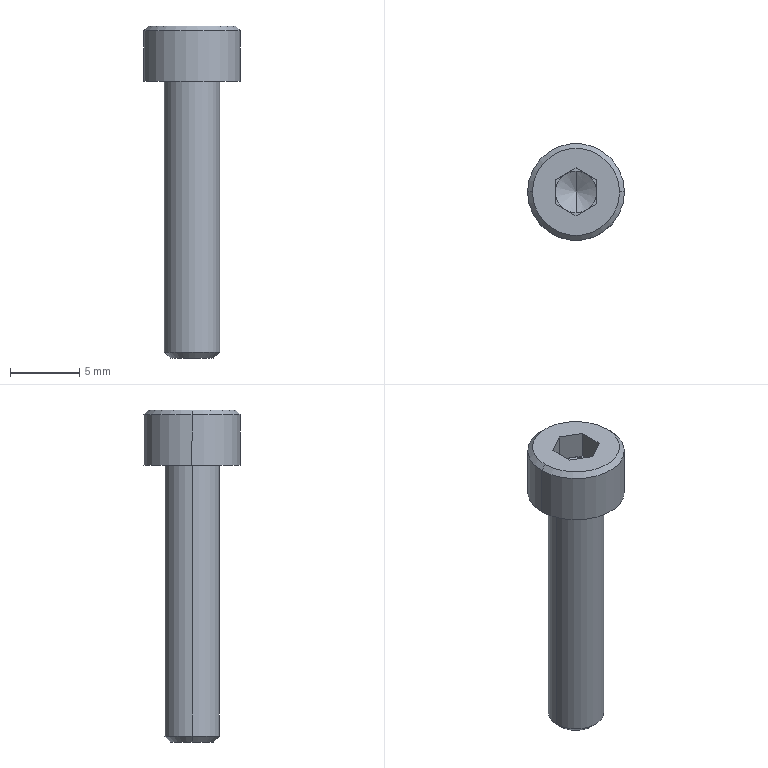Part | NX | features BREP 1 | 1 solid | 25 faces | box 7 x 7 x 24 mm | volume 385.258 mm3 | plane 15 | cone 6 | cylinder 4 | commonest cylinder face diameters 4 x2 7 x2
STEP:
#1=CARTESIAN_POINT('',(0.,-1.5,2.));
#2=VERTEX_POINT('',#1);
#3=CARTESIAN_POINT('',(0.,0.,1.134));
#4=VERTEX_POINT('',#3);
#5=CARTESIAN_POINT('',(0.,0.,1.134));
#6=DIRECTION('',(0.,-0.866,0.5));
#7=VECTOR('',#6,1000.);
#8=LINE('',#5,#7);
#9=EDGE_CURVE('',#2,#4,#8,.F.);
#10=ORIENTED_EDGE('',*,*,#9,.T.);
#11=CARTESIAN_POINT('',(0.,1.5,2.));
#12=VERTEX_POINT('',#11);
#13=CARTESIAN_POINT('',(0.,0.,1.134));
#14=DIRECTION('',(0.,0.866,0.5));
#15=VECTOR('',#14,1000.);
#16=LINE('',#13,#15);
#17=EDGE_CURVE('',#12,#4,#16,.F.);
#18=ORIENTED_EDGE('',*,*,#17,.F.);
#19=CARTESIAN_POINT('',(-0.75,1.299,2.));
#20=VERTEX_POINT('',#19);
#21=CARTESIAN_POINT('',(0.,0.,2.));
#22=DIRECTION('',(0.,0.,1.));
#23=DIRECTION('',(0.,-1.,0.));
#24=AXIS2_PLACEMENT_3D('',#21,#22,#23);
#25=CIRCLE('',#24,1.5);
#26=EDGE_CURVE('',#12,#20,#25,.T.);
#27=ORIENTED_EDGE('',*,*,#26,.T.);
#28=CARTESIAN_POINT('',(-1.5,0.,2.));
#29=VERTEX_POINT('',#28);
#30=CARTESIAN_POINT('',(0.,0.,2.));
#31=DIRECTION('',(0.,0.,1.));
#32=DIRECTION('',(0.,-1.,0.));
#33=AXIS2_PLACEMENT_3D('',#30,#31,#32);
#34=CIRCLE('',#33,1.5);
#35=EDGE_CURVE('',#20,#29,#34,.T.);
#36=ORIENTED_EDGE('',*,*,#35,.T.);
#37=CARTESIAN_POINT('',(-0.75,-1.299,2.));
#38=VERTEX_POINT('',#37);
#39=CARTESIAN_POINT('',(0.,0.,2.));
#40=DIRECTION('',(0.,0.,1.));
#41=DIRECTION('',(0.,-1.,0.));
#42=AXIS2_PLACEMENT_3D('',#39,#40,#41);
#43=CIRCLE('',#42,1.5);
#44=EDGE_CURVE('',#29,#38,#43,.T.);
#45=ORIENTED_EDGE('',*,*,#44,.T.);
#46=CARTESIAN_POINT('',(0.,0.,2.));
#47=DIRECTION('',(0.,0.,1.));
#48=DIRECTION('',(0.,-1.,0.));
#49=AXIS2_PLACEMENT_3D('',#46,#47,#48);
#50=CIRCLE('',#49,1.5);
#51=EDGE_CURVE('',#38,#2,#50,.T.);
#52=ORIENTED_EDGE('',*,*,#51,.T.);
#53=EDGE_LOOP('',(#10,#18,#27,#36,#45,#52));
#54=FACE_BOUND('',#53,.T.);
#55=CARTESIAN_POINT('',(0.,0.,1001.134));
#56=DIRECTION('',(0.,0.,1.));
#57=DIRECTION('',(0.,1.,0.));
#58=AXIS2_PLACEMENT_3D('',#55,#56,#57);
#59=CONICAL_SURFACE('',#58,1732.051,1.047);
#60=ADVANCED_FACE('',(#54),#59,.F.);
#61=CARTESIAN_POINT('',(3.5,0.,0.));
#62=VERTEX_POINT('',#61);
#63=CARTESIAN_POINT('',(-3.5,0.,0.));
#64=VERTEX_POINT('',#63);
#65=CARTESIAN_POINT('',(0.,0.,0.));
#66=DIRECTION('',(0.,0.,1.));
#67=DIRECTION('',(1.,0.,0.));
#68=AXIS2_PLACEMENT_3D('',#65,#66,#67);
#69=CIRCLE('',#68,3.5);
#70=EDGE_CURVE('',#62,#64,#69,.T.);
#71=ORIENTED_EDGE('',*,*,#70,.T.);
#72=CARTESIAN_POINT('',(-3.5,0.,3.65));
#73=VERTEX_POINT('',#72);
#74=CARTESIAN_POINT('',(-3.5,0.,0.));
#75=DIRECTION('',(0.,0.,1.));
#76=VECTOR('',#75,1000.);
#77=LINE('',#74,#76);
#78=EDGE_CURVE('',#64,#73,#77,.T.);
#79=ORIENTED_EDGE('',*,*,#78,.T.);
#80=CARTESIAN_POINT('',(3.5,0.,3.65));
#81=VERTEX_POINT('',#80);
#82=CARTESIAN_POINT('',(0.,0.,3.65));
#83=DIRECTION('',(0.,0.,1.));
#84=DIRECTION('',(1.,0.,0.));
#85=AXIS2_PLACEMENT_3D('',#82,#83,#84);
#86=CIRCLE('',#85,3.5);
#87=EDGE_CURVE('',#81,#73,#86,.T.);
#88=ORIENTED_EDGE('',*,*,#87,.F.);
#89=CARTESIAN_POINT('',(3.5,0.,0.));
#90=DIRECTION('',(0.,0.,1.));
#91=VECTOR('',#90,1000.);
#92=LINE('',#89,#91);
#93=EDGE_CURVE('',#62,#81,#92,.T.);
#94=ORIENTED_EDGE('',*,*,#93,.F.);
#95=EDGE_LOOP('',(#71,#79,#88,#94));
#96=FACE_BOUND('',#95,.T.);
#97=CARTESIAN_POINT('',(0.,0.,0.));
#98=DIRECTION('',(0.,0.,1.));
#99=DIRECTION('',(-1.,0.,0.));
#100=AXIS2_PLACEMENT_3D('',#97,#98,#99);
#101=CYLINDRICAL_SURFACE('',#100,3.5);
#102=ADVANCED_FACE('',(#96),#101,.T.);
#103=CARTESIAN_POINT('',(3.15,0.,4.));
#104=VERTEX_POINT('',#103);
#105=CARTESIAN_POINT('',(-3.15,0.,4.));
#106=VERTEX_POINT('',#105);
#107=CARTESIAN_POINT('',(0.,0.,4.));
#108=DIRECTION('',(0.,0.,1.));
#109=DIRECTION('',(1.,0.,0.));
#110=AXIS2_PLACEMENT_3D('',#107,#108,#109);
#111=CIRCLE('',#110,3.15);
#112=EDGE_CURVE('',#104,#106,#111,.T.);
#113=ORIENTED_EDGE('',*,*,#112,.F.);
#114=CARTESIAN_POINT('',(3.5,0.,3.65));
#115=DIRECTION('',(0.7071,0.,-0.7071));
#116=VECTOR('',#115,1000.);
#117=LINE('',#114,#116);
#118=EDGE_CURVE('',#81,#104,#117,.F.);
#119=ORIENTED_EDGE('',*,*,#118,.F.);
#120=ORIENTED_EDGE('',*,*,#87,.T.);
#121=CARTESIAN_POINT('',(-3.5,0.,3.65));
#122=DIRECTION('',(-0.7071,0.,-0.7071));
#123=VECTOR('',#122,1000.);
#124=LINE('',#121,#123);
#125=EDGE_CURVE('',#73,#106,#124,.F.);
#126=ORIENTED_EDGE('',*,*,#125,.T.);
#127=EDGE_LOOP('',(#113,#119,#120,#126));
#128=FACE_BOUND('',#127,.T.);
#129=CARTESIAN_POINT('',(0.,0.,3.65));
#130=DIRECTION('',(0.,0.,-1.));
#131=DIRECTION('',(1.,0.,0.));
#132=AXIS2_PLACEMENT_3D('',#129,#130,#131);
#133=CONICAL_SURFACE('',#132,3.5,0.7854);
#134=ADVANCED_FACE('',(#128),#133,.T.);
#135=CARTESIAN_POINT('',(1.571,0.,-20.));
#136=VERTEX_POINT('',#135);
#137=CARTESIAN_POINT('',(-1.571,0.,-20.));
#138=VERTEX_POINT('',#137);
#139=CARTESIAN_POINT('',(0.,0.,-20.));
#140=DIRECTION('',(0.,0.,1.));
#141=DIRECTION('',(1.,0.,0.));
#142=AXIS2_PLACEMENT_3D('',#139,#140,#141);
#143=CIRCLE('',#142,1.571);
#144=EDGE_CURVE('',#136,#138,#143,.T.);
#145=ORIENTED_EDGE('',*,*,#144,.T.);
#146=CARTESIAN_POINT('',(-2.,0.,-19.57));
#147=VERTEX_POINT('',#146);
#148=CARTESIAN_POINT('',(-1.571,0.,-20.));
#149=DIRECTION('',(-0.7071,0.,0.7071));
#150=VECTOR('',#149,1000.);
#151=LINE('',#148,#150);
#152=EDGE_CURVE('',#138,#147,#151,.T.);
#153=ORIENTED_EDGE('',*,*,#152,.T.);
#154=CARTESIAN_POINT('',(2.,0.,-19.57));
#155=VERTEX_POINT('',#154);
#156=CARTESIAN_POINT('',(0.,0.,-19.57));
#157=DIRECTION('',(0.,0.,1.));
#158=DIRECTION('',(1.,0.,0.));
#159=AXIS2_PLACEMENT_3D('',#156,#157,#158);
#160=CIRCLE('',#159,2.);
#161=EDGE_CURVE('',#155,#147,#160,.T.);
#162=ORIENTED_EDGE('',*,*,#161,.F.);
#163=CARTESIAN_POINT('',(1.571,0.,-20.));
#164=DIRECTION('',(0.7071,0.,0.7071));
#165=VECTOR('',#164,1000.);
#166=LINE('',#163,#165);
#167=EDGE_CURVE('',#136,#155,#166,.T.);
#168=ORIENTED_EDGE('',*,*,#167,.F.);
#169=EDGE_LOOP('',(#145,#153,#162,#168));
#170=FACE_BOUND('',#169,.T.);
#171=CARTESIAN_POINT('',(0.,0.,-20.));
#172=DIRECTION('',(0.,0.,1.));
#173=DIRECTION('',(-1.,0.,0.));
#174=AXIS2_PLACEMENT_3D('',#171,#172,#173);
#175=CONICAL_SURFACE('',#174,1.571,0.7854);
#176=ADVANCED_FACE('',(#170),#175,.T.);
#177=ORIENTED_EDGE('',*,*,#161,.T.);
#178=CARTESIAN_POINT('',(-2.,0.,0.));
#179=VERTEX_POINT('',#178);
#180=CARTESIAN_POINT('',(-2.,0.,-20.));
#181=DIRECTION('',(0.,0.,1.));
#182=VECTOR('',#181,1000.);
#183=LINE('',#180,#182);
#184=EDGE_CURVE('',#147,#179,#183,.T.);
#185=ORIENTED_EDGE('',*,*,#184,.T.);
#186=CARTESIAN_POINT('',(2.,0.,0.));
#187=VERTEX_POINT('',#186);
#188=CARTESIAN_POINT('',(0.,0.,0.));
#189=DIRECTION('',(0.,0.,1.));
#190=DIRECTION('',(1.,0.,0.));
#191=AXIS2_PLACEMENT_3D('',#188,#189,#190);
#192=CIRCLE('',#191,2.);
#193=EDGE_CURVE('',#187,#179,#192,.T.);
#194=ORIENTED_EDGE('',*,*,#193,.F.);
#195=CARTESIAN_POINT('',(2.,0.,-20.));
#196=DIRECTION('',(0.,0.,1.));
#197=VECTOR('',#196,1000.);
#198=LINE('',#195,#197);
#199=EDGE_CURVE('',#155,#187,#198,.T.);
#200=ORIENTED_EDGE('',*,*,#199,.F.);
#201=EDGE_LOOP('',(#177,#185,#194,#200));
#202=FACE_BOUND('',#201,.T.);
#203=CARTESIAN_POINT('',(0.,0.,-20.));
#204=DIRECTION('',(0.,0.,1.));
#205=DIRECTION('',(-1.,0.,0.));
#206=AXIS2_PLACEMENT_3D('',#203,#204,#205);
#207=CYLINDRICAL_SURFACE('',#206,2.);
#208=ADVANCED_FACE('',(#202),#207,.T.);
#209=CARTESIAN_POINT('',(0.75,-1.299,2.));
#210=VERTEX_POINT('',#209);
#211=CARTESIAN_POINT('',(1.5,0.,2.));
#212=VERTEX_POINT('',#211);
#213=CARTESIAN_POINT('',(0.,0.,2.));
#214=DIRECTION('',(0.,0.,1.));
#215=DIRECTION('',(0.,-1.,0.));
#216=AXIS2_PLACEMENT_3D('',#213,#214,#215);
#217=CIRCLE('',#216,1.5);
#218=EDGE_CURVE('',#210,#212,#217,.T.);
#219=ORIENTED_EDGE('',*,*,#218,.F.);
#220=CARTESIAN_POINT('',(1.5,-0.866,2.));
#221=VERTEX_POINT('',#220);
#222=CARTESIAN_POINT('',(0.,-1.732,2.));
#223=DIRECTION('',(0.866,0.5,0.));
#224=VECTOR('',#223,1000.);
#225=LINE('',#222,#224);
#226=EDGE_CURVE('',#210,#221,#225,.T.);
#227=ORIENTED_EDGE('',*,*,#226,.T.);
#228=CARTESIAN_POINT('',(1.5,-0.866,2.));
#229=DIRECTION('',(0.,1.,0.));
#230=VECTOR('',#229,1000.);
#231=LINE('',#228,#230);
#232=EDGE_CURVE('',#221,#212,#231,.T.);
#233=ORIENTED_EDGE('',*,*,#232,.T.);
#234=EDGE_LOOP('',(#219,#227,#233));
#235=FACE_BOUND('',#234,.T.);
#236=CARTESIAN_POINT('',(0.,0.,2.));
#237=DIRECTION('',(0.,0.,1.));
#238=DIRECTION('',(-1.,0.,0.));
#239=AXIS2_PLACEMENT_3D('',#236,#237,#238);
#240=PLANE('',#239);
#241=ADVANCED_FACE('',(#235),#240,.T.);
#242=CARTESIAN_POINT('',(0.75,1.299,2.));
#243=VERTEX_POINT('',#242);
#244=CARTESIAN_POINT('',(0.,0.,2.));
#245=DIRECTION('',(0.,0.,1.));
#246=DIRECTION('',(0.,-1.,0.));
#247=AXIS2_PLACEMENT_3D('',#244,#245,#246);
#248=CIRCLE('',#247,1.5);
#249=EDGE_CURVE('',#212,#243,#248,.T.);
#250=ORIENTED_EDGE('',*,*,#249,.F.);
#251=CARTESIAN_POINT('',(1.5,0.866,2.));
#252=VERTEX_POINT('',#251);
#253=CARTESIAN_POINT('',(1.5,-0.866,2.));
#254=DIRECTION('',(0.,1.,0.));
#255=VECTOR('',#254,1000.);
#256=LINE('',#253,#255);
#257=EDGE_CURVE('',#212,#252,#256,.T.);
#258=ORIENTED_EDGE('',*,*,#257,.T.);
#259=CARTESIAN_POINT('',(1.5,0.866,2.));
#260=DIRECTION('',(-0.866,0.5,0.));
#261=VECTOR('',#260,1000.);
#262=LINE('',#259,#261);
#263=EDGE_CURVE('',#252,#243,#262,.T.);
#264=ORIENTED_EDGE('',*,*,#263,.T.);
#265=EDGE_LOOP('',(#250,#258,#264));
#266=FACE_BOUND('',#265,.T.);
#267=CARTESIAN_POINT('',(0.,0.,2.));
#268=DIRECTION('',(0.,0.,1.));
#269=DIRECTION('',(-1.,0.,0.));
#270=AXIS2_PLACEMENT_3D('',#267,#268,#269);
#271=PLANE('',#270);
#272=ADVANCED_FACE('',(#266),#271,.T.);
#273=CARTESIAN_POINT('',(0.,0.,2.));
#274=DIRECTION('',(0.,0.,1.));
#275=DIRECTION('',(0.,-1.,0.));
#276=AXIS2_PLACEMENT_3D('',#273,#274,#275);
#277=CIRCLE('',#276,1.5);
#278=EDGE_CURVE('',#243,#12,#277,.T.);
#279=ORIENTED_EDGE('',*,*,#278,.F.);
#280=CARTESIAN_POINT('',(0.,1.732,2.));
#281=VERTEX_POINT('',#280);
#282=CARTESIAN_POINT('',(1.5,0.866,2.));
#283=DIRECTION('',(-0.866,0.5,0.));
#284=VECTOR('',#283,1000.);
#285=LINE('',#282,#284);
#286=EDGE_CURVE('',#243,#281,#285,.T.);
#287=ORIENTED_EDGE('',*,*,#286,.T.);
#288=CARTESIAN_POINT('',(0.,1.732,2.));
#289=DIRECTION('',(-0.866,-0.5,0.));
#290=VECTOR('',#289,1000.);
#291=LINE('',#288,#290);
#292=EDGE_CURVE('',#281,#20,#291,.T.);
#293=ORIENTED_EDGE('',*,*,#292,.T.);
#294=ORIENTED_EDGE('',*,*,#26,.F.);
#295=EDGE_LOOP('',(#279,#287,#293,#294));
#296=FACE_BOUND('',#295,.T.);
#297=CARTESIAN_POINT('',(0.,0.,2.));
#298=DIRECTION('',(0.,0.,1.));
#299=DIRECTION('',(-1.,0.,0.));
#300=AXIS2_PLACEMENT_3D('',#297,#298,#299);
#301=PLANE('',#300);
#302=ADVANCED_FACE('',(#296),#301,.T.);
#303=ORIENTED_EDGE('',*,*,#35,.F.);
#304=CARTESIAN_POINT('',(-1.5,0.866,2.));
#305=VERTEX_POINT('',#304);
#306=CARTESIAN_POINT('',(0.,1.732,2.));
#307=DIRECTION('',(-0.866,-0.5,0.));
#308=VECTOR('',#307,1000.);
#309=LINE('',#306,#308);
#310=EDGE_CURVE('',#20,#305,#309,.T.);
#311=ORIENTED_EDGE('',*,*,#310,.T.);
#312=CARTESIAN_POINT('',(-1.5,0.866,2.));
#313=DIRECTION('',(0.,-1.,0.));
#314=VECTOR('',#313,1000.);
#315=LINE('',#312,#314);
#316=EDGE_CURVE('',#305,#29,#315,.T.);
#317=ORIENTED_EDGE('',*,*,#316,.T.);
#318=EDGE_LOOP('',(#303,#311,#317));
#319=FACE_BOUND('',#318,.T.);
#320=CARTESIAN_POINT('',(0.,0.,2.));
#321=DIRECTION('',(0.,0.,1.));
#322=DIRECTION('',(-1.,0.,0.));
#323=AXIS2_PLACEMENT_3D('',#320,#321,#322);
#324=PLANE('',#323);
#325=ADVANCED_FACE('',(#319),#324,.T.);
#326=ORIENTED_EDGE('',*,*,#44,.F.);
#327=CARTESIAN_POINT('',(-1.5,-0.866,2.));
#328=VERTEX_POINT('',#327);
#329=CARTESIAN_POINT('',(-1.5,0.866,2.));
#330=DIRECTION('',(0.,-1.,0.));
#331=VECTOR('',#330,1000.);
#332=LINE('',#329,#331);
#333=EDGE_CURVE('',#29,#328,#332,.T.);
#334=ORIENTED_EDGE('',*,*,#333,.T.);
#335=CARTESIAN_POINT('',(-1.5,-0.866,2.));
#336=DIRECTION('',(0.866,-0.5,0.));
#337=VECTOR('',#336,1000.);
#338=LINE('',#335,#337);
#339=EDGE_CURVE('',#328,#38,#338,.T.);
#340=ORIENTED_EDGE('',*,*,#339,.T.);
#341=EDGE_LOOP('',(#326,#334,#340));
#342=FACE_BOUND('',#341,.T.);
#343=CARTESIAN_POINT('',(0.,0.,2.));
#344=DIRECTION('',(0.,0.,1.));
#345=DIRECTION('',(-1.,0.,0.));
#346=AXIS2_PLACEMENT_3D('',#343,#344,#345);
#347=PLANE('',#346);
#348=ADVANCED_FACE('',(#342),#347,.T.);
#349=ORIENTED_EDGE('',*,*,#184,.F.);
#350=CARTESIAN_POINT('',(0.,0.,-19.57));
#351=DIRECTION('',(0.,0.,1.));
#352=DIRECTION('',(1.,0.,0.));
#353=AXIS2_PLACEMENT_3D('',#350,#351,#352);
#354=CIRCLE('',#353,2.);
#355=EDGE_CURVE('',#147,#155,#354,.T.);
#356=ORIENTED_EDGE('',*,*,#355,.T.);
#357=ORIENTED_EDGE('',*,*,#199,.T.);
#358=CARTESIAN_POINT('',(0.,0.,0.));
#359=DIRECTION('',(0.,0.,1.));
#360=DIRECTION('',(1.,0.,0.));
#361=AXIS2_PLACEMENT_3D('',#358,#359,#360);
#362=CIRCLE('',#361,2.);
#363=EDGE_CURVE('',#179,#187,#362,.T.);
#364=ORIENTED_EDGE('',*,*,#363,.F.);
#365=EDGE_LOOP('',(#349,#356,#357,#364));
#366=FACE_BOUND('',#365,.T.);
#367=CARTESIAN_POINT('',(0.,0.,-20.));
#368=DIRECTION('',(0.,0.,1.));
#369=DIRECTION('',(-1.,0.,0.));
#370=AXIS2_PLACEMENT_3D('',#367,#368,#369);
#371=CYLINDRICAL_SURFACE('',#370,2.);
#372=ADVANCED_FACE('',(#366),#371,.T.);
#373=ORIENTED_EDGE('',*,*,#152,.F.);
#374=CARTESIAN_POINT('',(0.,0.,-20.));
#375=DIRECTION('',(0.,0.,1.));
#376=DIRECTION('',(1.,0.,0.));
#377=AXIS2_PLACEMENT_3D('',#374,#375,#376);
#378=CIRCLE('',#377,1.571);
#379=EDGE_CURVE('',#138,#136,#378,.T.);
#380=ORIENTED_EDGE('',*,*,#379,.T.);
#381=ORIENTED_EDGE('',*,*,#167,.T.);
#382=ORIENTED_EDGE('',*,*,#355,.F.);
#383=EDGE_LOOP('',(#373,#380,#381,#382));
#384=FACE_BOUND('',#383,.T.);
#385=CARTESIAN_POINT('',(0.,0.,-20.));
#386=DIRECTION('',(0.,0.,1.));
#387=DIRECTION('',(-1.,0.,0.));
#388=AXIS2_PLACEMENT_3D('',#385,#386,#387);
#389=CONICAL_SURFACE('',#388,1.571,0.7854);
#390=ADVANCED_FACE('',(#384),#389,.T.);
#391=ORIENTED_EDGE('',*,*,#144,.F.);
#392=ORIENTED_EDGE('',*,*,#379,.F.);
#393=EDGE_LOOP('',(#391,#392));
#394=FACE_BOUND('',#393,.T.);
#395=CARTESIAN_POINT('',(0.,1.571,-20.));
#396=DIRECTION('',(0.,0.,1.));
#397=DIRECTION('',(-1.,0.,0.));
#398=AXIS2_PLACEMENT_3D('',#395,#396,#397);
#399=PLANE('',#398);
#400=ADVANCED_FACE('',(#394),#399,.F.);
#401=CARTESIAN_POINT('',(0.,-1.732,4.));
#402=VERTEX_POINT('',#401);
#403=CARTESIAN_POINT('',(1.5,-0.866,4.));
#404=VERTEX_POINT('',#403);
#405=CARTESIAN_POINT('',(0.,-1.732,4.));
#406=DIRECTION('',(0.866,0.5,0.));
#407=VECTOR('',#406,1000.);
#408=LINE('',#405,#407);
#409=EDGE_CURVE('',#402,#404,#408,.T.);
#410=ORIENTED_EDGE('',*,*,#409,.F.);
#411=CARTESIAN_POINT('',(-1.5,-0.866,4.));
#412=VERTEX_POINT('',#411);
#413=CARTESIAN_POINT('',(-1.5,-0.866,4.));
#414=DIRECTION('',(0.866,-0.5,0.));
#415=VECTOR('',#414,1000.);
#416=LINE('',#413,#415);
#417=EDGE_CURVE('',#412,#402,#416,.T.);
#418=ORIENTED_EDGE('',*,*,#417,.F.);
#419=CARTESIAN_POINT('',(-1.5,0.866,4.));
#420=VERTEX_POINT('',#419);
#421=CARTESIAN_POINT('',(-1.5,0.866,4.));
#422=DIRECTION('',(0.,-1.,0.));
#423=VECTOR('',#422,1000.);
#424=LINE('',#421,#423);
#425=EDGE_CURVE('',#420,#412,#424,.T.);
#426=ORIENTED_EDGE('',*,*,#425,.F.);
#427=CARTESIAN_POINT('',(0.,1.732,4.));
#428=VERTEX_POINT('',#427);
#429=CARTESIAN_POINT('',(0.,1.732,4.));
#430=DIRECTION('',(-0.866,-0.5,0.));
#431=VECTOR('',#430,1000.);
#432=LINE('',#429,#431);
#433=EDGE_CURVE('',#428,#420,#432,.T.);
#434=ORIENTED_EDGE('',*,*,#433,.F.);
#435=CARTESIAN_POINT('',(1.5,0.866,4.));
#436=VERTEX_POINT('',#435);
#437=CARTESIAN_POINT('',(1.5,0.866,4.));
#438=DIRECTION('',(-0.866,0.5,0.));
#439=VECTOR('',#438,1000.);
#440=LINE('',#437,#439);
#441=EDGE_CURVE('',#436,#428,#440,.T.);
#442=ORIENTED_EDGE('',*,*,#441,.F.);
#443=CARTESIAN_POINT('',(1.5,-0.866,4.));
#444=DIRECTION('',(0.,1.,0.));
#445=VECTOR('',#444,1000.);
#446=LINE('',#443,#445);
#447=EDGE_CURVE('',#404,#436,#446,.T.);
#448=ORIENTED_EDGE('',*,*,#447,.F.);
#449=EDGE_LOOP('',(#410,#418,#426,#434,#442,#448));
#450=FACE_BOUND('',#449,.T.);
#451=CARTESIAN_POINT('',(0.,0.,4.));
#452=DIRECTION('',(0.,0.,1.));
#453=DIRECTION('',(1.,0.,0.));
#454=AXIS2_PLACEMENT_3D('',#451,#452,#453);
#455=CIRCLE('',#454,3.15);
#456=EDGE_CURVE('',#106,#104,#455,.T.);
#457=ORIENTED_EDGE('',*,*,#456,.T.);
#458=ORIENTED_EDGE('',*,*,#112,.T.);
#459=EDGE_LOOP('',(#457,#458));
#460=FACE_BOUND('',#459,.T.);
#461=CARTESIAN_POINT('',(0.,0.,4.));
#462=DIRECTION('',(0.,0.,-1.));
#463=DIRECTION('',(1.,0.,0.));
#464=AXIS2_PLACEMENT_3D('',#461,#462,#463);
#465=PLANE('',#464);
#466=ADVANCED_FACE('',(#450,#460),#465,.F.);
#467=ORIENTED_EDGE('',*,*,#118,.T.);
#468=ORIENTED_EDGE('',*,*,#456,.F.);
#469=ORIENTED_EDGE('',*,*,#125,.F.);
#470=CARTESIAN_POINT('',(0.,0.,3.65));
#471=DIRECTION('',(0.,0.,1.));
#472=DIRECTION('',(1.,0.,0.));
#473=AXIS2_PLACEMENT_3D('',#470,#471,#472);
#474=CIRCLE('',#473,3.5);
#475=EDGE_CURVE('',#73,#81,#474,.T.);
#476=ORIENTED_EDGE('',*,*,#475,.T.);
#477=EDGE_LOOP('',(#467,#468,#469,#476));
#478=FACE_BOUND('',#477,.T.);
#479=CARTESIAN_POINT('',(0.,0.,3.65));
#480=DIRECTION('',(0.,0.,-1.));
#481=DIRECTION('',(1.,0.,0.));
#482=AXIS2_PLACEMENT_3D('',#479,#480,#481);
#483=CONICAL_SURFACE('',#482,3.5,0.7854);
#484=ADVANCED_FACE('',(#478),#483,.T.);
#485=ORIENTED_EDGE('',*,*,#78,.F.);
#486=CARTESIAN_POINT('',(0.,0.,0.));
#487=DIRECTION('',(0.,0.,1.));
#488=DIRECTION('',(1.,0.,0.));
#489=AXIS2_PLACEMENT_3D('',#486,#487,#488);
#490=CIRCLE('',#489,3.5);
#491=EDGE_CURVE('',#64,#62,#490,.T.);
#492=ORIENTED_EDGE('',*,*,#491,.T.);
#493=ORIENTED_EDGE('',*,*,#93,.T.);
#494=ORIENTED_EDGE('',*,*,#475,.F.);
#495=EDGE_LOOP('',(#485,#492,#493,#494));
#496=FACE_BOUND('',#495,.T.);
#497=CARTESIAN_POINT('',(0.,0.,0.));
#498=DIRECTION('',(0.,0.,1.));
#499=DIRECTION('',(-1.,0.,0.));
#500=AXIS2_PLACEMENT_3D('',#497,#498,#499);
#501=CYLINDRICAL_SURFACE('',#500,3.5);
#502=ADVANCED_FACE('',(#496),#501,.T.);
#503=ORIENTED_EDGE('',*,*,#193,.T.);
#504=ORIENTED_EDGE('',*,*,#363,.T.);
#505=EDGE_LOOP('',(#503,#504));
#506=FACE_BOUND('',#505,.T.);
#507=ORIENTED_EDGE('',*,*,#70,.F.);
#508=ORIENTED_EDGE('',*,*,#491,.F.);
#509=EDGE_LOOP('',(#507,#508));
#510=FACE_BOUND('',#509,.T.);
#511=CARTESIAN_POINT('',(0.,3.5,0.));
#512=DIRECTION('',(0.,0.,1.));
#513=DIRECTION('',(-1.,0.,0.));
#514=AXIS2_PLACEMENT_3D('',#511,#512,#513);
#515=PLANE('',#514);
#516=ADVANCED_FACE('',(#506,#510),#515,.F.);
#517=ORIENTED_EDGE('',*,*,#417,.T.);
#518=CARTESIAN_POINT('',(0.,-1.732,2.));
#519=VERTEX_POINT('',#518);
#520=CARTESIAN_POINT('',(0.,-1.732,2.));
#521=DIRECTION('',(0.,0.,1.));
#522=VECTOR('',#521,1000.);
#523=LINE('',#520,#522);
#524=EDGE_CURVE('',#519,#402,#523,.T.);
#525=ORIENTED_EDGE('',*,*,#524,.F.);
#526=CARTESIAN_POINT('',(-1.5,-0.866,2.));
#527=DIRECTION('',(0.866,-0.5,0.));
#528=VECTOR('',#527,1000.);
#529=LINE('',#526,#528);
#530=EDGE_CURVE('',#38,#519,#529,.T.);
#531=ORIENTED_EDGE('',*,*,#530,.F.);
#532=ORIENTED_EDGE('',*,*,#339,.F.);
#533=CARTESIAN_POINT('',(-1.5,-0.866,2.));
#534=DIRECTION('',(0.,0.,1.));
#535=VECTOR('',#534,1000.);
#536=LINE('',#533,#535);
#537=EDGE_CURVE('',#328,#412,#536,.T.);
#538=ORIENTED_EDGE('',*,*,#537,.T.);
#539=EDGE_LOOP('',(#517,#525,#531,#532,#538));
#540=FACE_BOUND('',#539,.T.);
#541=CARTESIAN_POINT('',(-1.5,-0.866,2.));
#542=DIRECTION('',(-0.5,-0.866,0.));
#543=DIRECTION('',(-0.866,0.5,0.));
#544=AXIS2_PLACEMENT_3D('',#541,#542,#543);
#545=PLANE('',#544);
#546=ADVANCED_FACE('',(#540),#545,.F.);
#547=ORIENTED_EDGE('',*,*,#425,.T.);
#548=ORIENTED_EDGE('',*,*,#537,.F.);
#549=ORIENTED_EDGE('',*,*,#333,.F.);
#550=ORIENTED_EDGE('',*,*,#316,.F.);
#551=CARTESIAN_POINT('',(-1.5,0.866,2.));
#552=DIRECTION('',(0.,0.,1.));
#553=VECTOR('',#552,1000.);
#554=LINE('',#551,#553);
#555=EDGE_CURVE('',#305,#420,#554,.T.);
#556=ORIENTED_EDGE('',*,*,#555,.T.);
#557=EDGE_LOOP('',(#547,#548,#549,#550,#556));
#558=FACE_BOUND('',#557,.T.);
#559=CARTESIAN_POINT('',(-1.5,0.866,2.));
#560=DIRECTION('',(-1.,0.,0.));
#561=DIRECTION('',(0.,0.,-1.));
#562=AXIS2_PLACEMENT_3D('',#559,#560,#561);
#563=PLANE('',#562);
#564=ADVANCED_FACE('',(#558),#563,.F.);
#565=ORIENTED_EDGE('',*,*,#433,.T.);
#566=ORIENTED_EDGE('',*,*,#555,.F.);
#567=ORIENTED_EDGE('',*,*,#310,.F.);
#568=ORIENTED_EDGE('',*,*,#292,.F.);
#569=CARTESIAN_POINT('',(0.,1.732,2.));
#570=DIRECTION('',(0.,0.,1.));
#571=VECTOR('',#570,1000.);
#572=LINE('',#569,#571);
#573=EDGE_CURVE('',#281,#428,#572,.T.);
#574=ORIENTED_EDGE('',*,*,#573,.T.);
#575=EDGE_LOOP('',(#565,#566,#567,#568,#574));
#576=FACE_BOUND('',#575,.T.);
#577=CARTESIAN_POINT('',(0.,1.732,2.));
#578=DIRECTION('',(-0.5,0.866,0.));
#579=DIRECTION('',(0.866,0.5,0.));
#580=AXIS2_PLACEMENT_3D('',#577,#578,#579);
#581=PLANE('',#580);
#582=ADVANCED_FACE('',(#576),#581,.F.);
#583=ORIENTED_EDGE('',*,*,#441,.T.);
#584=ORIENTED_EDGE('',*,*,#573,.F.);
#585=ORIENTED_EDGE('',*,*,#286,.F.);
#586=ORIENTED_EDGE('',*,*,#263,.F.);
#587=CARTESIAN_POINT('',(1.5,0.866,2.));
#588=DIRECTION('',(0.,0.,1.));
#589=VECTOR('',#588,1000.);
#590=LINE('',#587,#589);
#591=EDGE_CURVE('',#252,#436,#590,.T.);
#592=ORIENTED_EDGE('',*,*,#591,.T.);
#593=EDGE_LOOP('',(#583,#584,#585,#586,#592));
#594=FACE_BOUND('',#593,.T.);
#595=CARTESIAN_POINT('',(1.5,0.866,2.));
#596=DIRECTION('',(0.5,0.866,0.));
#597=DIRECTION('',(0.866,-0.5,0.));
#598=AXIS2_PLACEMENT_3D('',#595,#596,#597);
#599=PLANE('',#598);
#600=ADVANCED_FACE('',(#594),#599,.F.);
#601=ORIENTED_EDGE('',*,*,#447,.T.);
#602=ORIENTED_EDGE('',*,*,#591,.F.);
#603=ORIENTED_EDGE('',*,*,#257,.F.);
#604=ORIENTED_EDGE('',*,*,#232,.F.);
#605=CARTESIAN_POINT('',(1.5,-0.866,2.));
#606=DIRECTION('',(0.,0.,1.));
#607=VECTOR('',#606,1000.);
#608=LINE('',#605,#607);
#609=EDGE_CURVE('',#221,#404,#608,.T.);
#610=ORIENTED_EDGE('',*,*,#609,.T.);
#611=EDGE_LOOP('',(#601,#602,#603,#604,#610));
#612=FACE_BOUND('',#611,.T.);
#613=CARTESIAN_POINT('',(1.5,-0.866,2.));
#614=DIRECTION('',(1.,0.,0.));
#615=DIRECTION('',(0.,0.,1.));
#616=AXIS2_PLACEMENT_3D('',#613,#614,#615);
#617=PLANE('',#616);
#618=ADVANCED_FACE('',(#612),#617,.F.);
#619=ORIENTED_EDGE('',*,*,#409,.T.);
#620=ORIENTED_EDGE('',*,*,#609,.F.);
#621=ORIENTED_EDGE('',*,*,#226,.F.);
#622=CARTESIAN_POINT('',(0.,-1.732,2.));
#623=DIRECTION('',(0.866,0.5,0.));
#624=VECTOR('',#623,1000.);
#625=LINE('',#622,#624);
#626=EDGE_CURVE('',#519,#210,#625,.T.);
#627=ORIENTED_EDGE('',*,*,#626,.F.);
#628=ORIENTED_EDGE('',*,*,#524,.T.);
#629=EDGE_LOOP('',(#619,#620,#621,#627,#628));
#630=FACE_BOUND('',#629,.T.);
#631=CARTESIAN_POINT('',(0.,-1.732,2.));
#632=DIRECTION('',(0.5,-0.866,0.));
#633=DIRECTION('',(-0.866,-0.5,0.));
#634=AXIS2_PLACEMENT_3D('',#631,#632,#633);
#635=PLANE('',#634);
#636=ADVANCED_FACE('',(#630),#635,.F.);
#637=ORIENTED_EDGE('',*,*,#51,.F.);
#638=ORIENTED_EDGE('',*,*,#530,.T.);
#639=ORIENTED_EDGE('',*,*,#626,.T.);
#640=CARTESIAN_POINT('',(0.,0.,2.));
#641=DIRECTION('',(0.,0.,1.));
#642=DIRECTION('',(0.,-1.,0.));
#643=AXIS2_PLACEMENT_3D('',#640,#641,#642);
#644=CIRCLE('',#643,1.5);
#645=EDGE_CURVE('',#2,#210,#644,.T.);
#646=ORIENTED_EDGE('',*,*,#645,.F.);
#647=EDGE_LOOP('',(#637,#638,#639,#646));
#648=FACE_BOUND('',#647,.T.);
#649=CARTESIAN_POINT('',(0.,0.,2.));
#650=DIRECTION('',(0.,0.,1.));
#651=DIRECTION('',(-1.,0.,0.));
#652=AXIS2_PLACEMENT_3D('',#649,#650,#651);
#653=PLANE('',#652);
#654=ADVANCED_FACE('',(#648),#653,.T.);
#655=ORIENTED_EDGE('',*,*,#17,.T.);
#656=ORIENTED_EDGE('',*,*,#9,.F.);
#657=ORIENTED_EDGE('',*,*,#645,.T.);
#658=ORIENTED_EDGE('',*,*,#218,.T.);
#659=ORIENTED_EDGE('',*,*,#249,.T.);
#660=ORIENTED_EDGE('',*,*,#278,.T.);
#661=EDGE_LOOP('',(#655,#656,#657,#658,#659,#660));
#662=FACE_BOUND('',#661,.T.);
#663=CARTESIAN_POINT('',(0.,0.,1001.134));
#664=DIRECTION('',(0.,0.,1.));
#665=DIRECTION('',(0.,1.,0.));
#666=AXIS2_PLACEMENT_3D('',#663,#664,#665);
#667=CONICAL_SURFACE('',#666,1732.051,1.047);
#668=ADVANCED_FACE('',(#662),#667,.F.);
#669=CLOSED_SHELL('',(#60,#102,#134,#176,#208,#241,#272,#302,#325,#348,#372,#390,#400,#466,#484,#502,#516,#546,#564,#582,#600,#618,#636,#654,#668));
#670=MANIFOLD_SOLID_BREP('',#669);
#671=(LENGTH_UNIT()NAMED_UNIT(*)SI_UNIT(.MILLI.,.METRE.));
#672=UNCERTAINTY_MEASURE_WITH_UNIT(LENGTH_MEASURE(0.00001),#671,'','');
#673=(NAMED_UNIT(*)PLANE_ANGLE_UNIT()SI_UNIT($,.RADIAN.));
#674=(NAMED_UNIT(*)SI_UNIT($,.STERADIAN.)SOLID_ANGLE_UNIT());
#675=(GEOMETRIC_REPRESENTATION_CONTEXT(3)GLOBAL_UNCERTAINTY_ASSIGNED_CONTEXT((#672))GLOBAL_UNIT_ASSIGNED_CONTEXT((#671,#673,#674))REPRESENTATION_CONTEXT('',''));
#676=ADVANCED_BREP_SHAPE_REPRESENTATION('',(#670),#675);